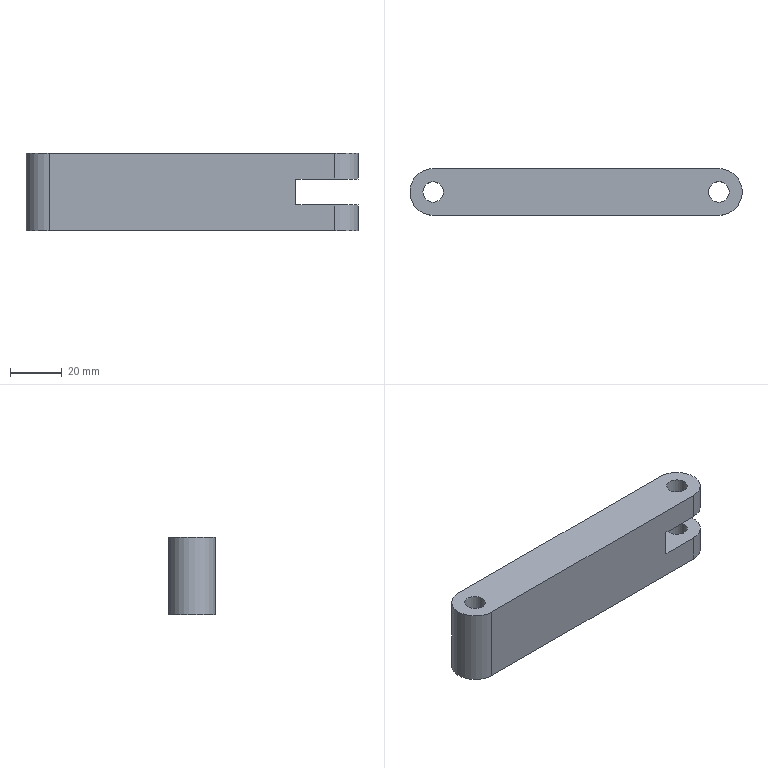Part | STEP file | 1 solid | 13 faces | box 128 x 18 x 30 mm | volume 60581 mm3 | plane 7 | cylinder 6 | commonest cylinder face diameters 18 x3 8 x2 7.914 x1
STEP:
#1=CARTESIAN_POINT('',(0.,0.,0.));
#2=DIRECTION('',(0.,0.,1.));
#3=DIRECTION('',(1.,0.,0.));
#4=AXIS2_PLACEMENT_3D('',#1,#2,#3);
#5=CARTESIAN_POINT('',(40.,-9.,-5.));
#6=VERTEX_POINT('',#5);
#7=CARTESIAN_POINT('',(55.,-9.,-5.));
#8=VERTEX_POINT('',#7);
#9=CARTESIAN_POINT('',(-55.,-9.,-5.));
#10=DIRECTION('',(1.,0.,0.));
#11=VECTOR('',#10,1.);
#12=LINE('',#9,#11);
#13=CARTESIAN_POINT('',(-55.,-9.,15.));
#14=DIRECTION('',(0.,1.,0.));
#15=DIRECTION('',(0.,0.,1.));
#16=AXIS2_PLACEMENT_3D('',#13,#14,#15);
#17=PLANE('',#16);
#18=CARTESIAN_POINT('',(-20.,0.));
#19=DIRECTION('',(0.,1.));
#20=VECTOR('',#19,1.);
#21=LINE('',#18,#20);
#22=(GEOMETRIC_REPRESENTATION_CONTEXT(2)PARAMETRIC_REPRESENTATION_CONTEXT()REPRESENTATION_CONTEXT('',''));
#23=DEFINITIONAL_REPRESENTATION('',(#21),#22);
#24=PCURVE('',#17,#23);
#25=CARTESIAN_POINT('',(0.,0.,-5.));
#26=DIRECTION('',(0.,0.,-1.));
#27=DIRECTION('',(-1.,0.,0.));
#28=AXIS2_PLACEMENT_3D('',#25,#26,#27);
#29=PLANE('',#28);
#30=CARTESIAN_POINT('',(55.,-9.));
#31=DIRECTION('',(-1.,0.));
#32=VECTOR('',#31,1.);
#33=LINE('',#30,#32);
#34=(GEOMETRIC_REPRESENTATION_CONTEXT(2)PARAMETRIC_REPRESENTATION_CONTEXT()REPRESENTATION_CONTEXT('',''));
#35=DEFINITIONAL_REPRESENTATION('',(#33),#34);
#36=PCURVE('',#29,#35);
#37=SURFACE_CURVE('',#12,(#24,#36),.PCURVE_S1.);
#38=EDGE_CURVE('',#6,#8,#37,.T.);
#39=ORIENTED_EDGE('',*,*,#38,.F.);
#40=CARTESIAN_POINT('',(40.,-9.,5.));
#41=VERTEX_POINT('',#40);
#42=CARTESIAN_POINT('',(40.,-9.,15.));
#43=DIRECTION('',(0.,0.,-1.));
#44=VECTOR('',#43,1.);
#45=LINE('',#42,#44);
#46=CARTESIAN_POINT('',(0.,95.));
#47=DIRECTION('',(-1.,0.));
#48=VECTOR('',#47,1.);
#49=LINE('',#46,#48);
#50=(GEOMETRIC_REPRESENTATION_CONTEXT(2)PARAMETRIC_REPRESENTATION_CONTEXT()REPRESENTATION_CONTEXT('',''));
#51=DEFINITIONAL_REPRESENTATION('',(#49),#50);
#52=PCURVE('',#17,#51);
#53=CARTESIAN_POINT('',(40.,-9.,-5.));
#54=DIRECTION('',(-1.,0.,0.));
#55=DIRECTION('',(0.,0.,1.));
#56=AXIS2_PLACEMENT_3D('',#53,#54,#55);
#57=PLANE('',#56);
#58=CARTESIAN_POINT('',(20.,0.));
#59=DIRECTION('',(-1.,0.));
#60=VECTOR('',#59,1.);
#61=LINE('',#58,#60);
#62=(GEOMETRIC_REPRESENTATION_CONTEXT(2)PARAMETRIC_REPRESENTATION_CONTEXT()REPRESENTATION_CONTEXT('',''));
#63=DEFINITIONAL_REPRESENTATION('',(#61),#62);
#64=PCURVE('',#57,#63);
#65=SURFACE_CURVE('',#45,(#52,#64),.PCURVE_S1.);
#66=EDGE_CURVE('',#41,#6,#65,.T.);
#67=ORIENTED_EDGE('',*,*,#66,.F.);
#68=CARTESIAN_POINT('',(55.,-9.,5.));
#69=VERTEX_POINT('',#68);
#70=CARTESIAN_POINT('',(-55.,-9.,5.));
#71=DIRECTION('',(-1.,0.,0.));
#72=VECTOR('',#71,1.);
#73=LINE('',#70,#72);
#74=CARTESIAN_POINT('',(-10.,0.));
#75=DIRECTION('',(0.,-1.));
#76=VECTOR('',#75,1.);
#77=LINE('',#74,#76);
#78=(GEOMETRIC_REPRESENTATION_CONTEXT(2)PARAMETRIC_REPRESENTATION_CONTEXT()REPRESENTATION_CONTEXT('',''));
#79=DEFINITIONAL_REPRESENTATION('',(#77),#78);
#80=PCURVE('',#17,#79);
#81=CARTESIAN_POINT('',(0.,0.,5.));
#82=DIRECTION('',(0.,0.,-1.));
#83=DIRECTION('',(-1.,0.,0.));
#84=AXIS2_PLACEMENT_3D('',#81,#82,#83);
#85=PLANE('',#84);
#86=CARTESIAN_POINT('',(55.,-9.));
#87=DIRECTION('',(1.,0.));
#88=VECTOR('',#87,1.);
#89=LINE('',#86,#88);
#90=(GEOMETRIC_REPRESENTATION_CONTEXT(2)PARAMETRIC_REPRESENTATION_CONTEXT()REPRESENTATION_CONTEXT('',''));
#91=DEFINITIONAL_REPRESENTATION('',(#89),#90);
#92=PCURVE('',#85,#91);
#93=SURFACE_CURVE('',#73,(#80,#92),.PCURVE_S1.);
#94=EDGE_CURVE('',#69,#41,#93,.T.);
#95=ORIENTED_EDGE('',*,*,#94,.F.);
#96=CARTESIAN_POINT('',(55.,-9.,15.));
#97=VERTEX_POINT('',#96);
#98=CARTESIAN_POINT('',(55.,-9.,15.));
#99=DIRECTION('',(0.,0.,-1.));
#100=VECTOR('',#99,1.);
#101=LINE('',#98,#100);
#102=CARTESIAN_POINT('',(0.,110.));
#103=DIRECTION('',(-1.,0.));
#104=VECTOR('',#103,1.);
#105=LINE('',#102,#104);
#106=(GEOMETRIC_REPRESENTATION_CONTEXT(2)PARAMETRIC_REPRESENTATION_CONTEXT()REPRESENTATION_CONTEXT('',''));
#107=DEFINITIONAL_REPRESENTATION('',(#105),#106);
#108=PCURVE('',#17,#107);
#109=CARTESIAN_POINT('',(55.,0.,15.));
#110=DIRECTION('',(0.,0.,-1.));
#111=DIRECTION('',(-1.,0.,0.));
#112=AXIS2_PLACEMENT_3D('',#109,#110,#111);
#113=CYLINDRICAL_SURFACE('',#112,9.);
#114=CARTESIAN_POINT('',(4.712,0.));
#115=DIRECTION('',(0.,1.));
#116=VECTOR('',#115,1.);
#117=LINE('',#114,#116);
#118=(GEOMETRIC_REPRESENTATION_CONTEXT(2)PARAMETRIC_REPRESENTATION_CONTEXT()REPRESENTATION_CONTEXT('',''));
#119=DEFINITIONAL_REPRESENTATION('',(#117),#118);
#120=PCURVE('',#113,#119);
#121=SURFACE_CURVE('',#101,(#108,#120),.PCURVE_S1.);
#122=EDGE_CURVE('',#97,#69,#121,.T.);
#123=ORIENTED_EDGE('',*,*,#122,.F.);
#124=CARTESIAN_POINT('',(-55.,-9.,15.));
#125=VERTEX_POINT('',#124);
#126=CARTESIAN_POINT('',(-55.,-9.,15.));
#127=DIRECTION('',(1.,0.,0.));
#128=VECTOR('',#127,1.);
#129=LINE('',#126,#128);
#130=CARTESIAN_POINT('',(0.,0.));
#131=DIRECTION('',(0.,1.));
#132=VECTOR('',#131,1.);
#133=LINE('',#130,#132);
#134=(GEOMETRIC_REPRESENTATION_CONTEXT(2)PARAMETRIC_REPRESENTATION_CONTEXT()REPRESENTATION_CONTEXT('',''));
#135=DEFINITIONAL_REPRESENTATION('',(#133),#134);
#136=PCURVE('',#17,#135);
#137=CARTESIAN_POINT('',(-55.,0.,15.));
#138=DIRECTION('',(0.,0.,1.));
#139=DIRECTION('',(1.,0.,0.));
#140=AXIS2_PLACEMENT_3D('',#137,#138,#139);
#141=PLANE('',#140);
#142=CARTESIAN_POINT('',(0.,-9.));
#143=DIRECTION('',(1.,0.));
#144=VECTOR('',#143,1.);
#145=LINE('',#142,#144);
#146=(GEOMETRIC_REPRESENTATION_CONTEXT(2)PARAMETRIC_REPRESENTATION_CONTEXT()REPRESENTATION_CONTEXT('',''));
#147=DEFINITIONAL_REPRESENTATION('',(#145),#146);
#148=PCURVE('',#141,#147);
#149=SURFACE_CURVE('',#129,(#136,#148),.PCURVE_S1.);
#150=EDGE_CURVE('',#125,#97,#149,.T.);
#151=ORIENTED_EDGE('',*,*,#150,.F.);
#152=CARTESIAN_POINT('',(-55.,-9.,-15.));
#153=VERTEX_POINT('',#152);
#154=CARTESIAN_POINT('',(-55.,-9.,15.));
#155=DIRECTION('',(0.,0.,1.));
#156=VECTOR('',#155,1.);
#157=LINE('',#154,#156);
#158=CARTESIAN_POINT('',(0.,0.));
#159=DIRECTION('',(1.,0.));
#160=VECTOR('',#159,1.);
#161=LINE('',#158,#160);
#162=(GEOMETRIC_REPRESENTATION_CONTEXT(2)PARAMETRIC_REPRESENTATION_CONTEXT()REPRESENTATION_CONTEXT('',''));
#163=DEFINITIONAL_REPRESENTATION('',(#161),#162);
#164=PCURVE('',#17,#163);
#165=CARTESIAN_POINT('',(-55.,0.,15.));
#166=DIRECTION('',(0.,0.,-1.));
#167=DIRECTION('',(-1.,0.,0.));
#168=AXIS2_PLACEMENT_3D('',#165,#166,#167);
#169=CYLINDRICAL_SURFACE('',#168,9.);
#170=CARTESIAN_POINT('',(-1.571,0.));
#171=DIRECTION('',(0.,-1.));
#172=VECTOR('',#171,1.);
#173=LINE('',#170,#172);
#174=(GEOMETRIC_REPRESENTATION_CONTEXT(2)PARAMETRIC_REPRESENTATION_CONTEXT()REPRESENTATION_CONTEXT('',''));
#175=DEFINITIONAL_REPRESENTATION('',(#173),#174);
#176=PCURVE('',#169,#175);
#177=SURFACE_CURVE('',#157,(#164,#176),.PCURVE_S1.);
#178=EDGE_CURVE('',#153,#125,#177,.T.);
#179=ORIENTED_EDGE('',*,*,#178,.F.);
#180=CARTESIAN_POINT('',(55.,-9.,-15.));
#181=VERTEX_POINT('',#180);
#182=CARTESIAN_POINT('',(-55.,-9.,-15.));
#183=DIRECTION('',(-1.,0.,0.));
#184=VECTOR('',#183,1.);
#185=LINE('',#182,#184);
#186=CARTESIAN_POINT('',(-30.,0.));
#187=DIRECTION('',(0.,-1.));
#188=VECTOR('',#187,1.);
#189=LINE('',#186,#188);
#190=(GEOMETRIC_REPRESENTATION_CONTEXT(2)PARAMETRIC_REPRESENTATION_CONTEXT()REPRESENTATION_CONTEXT('',''));
#191=DEFINITIONAL_REPRESENTATION('',(#189),#190);
#192=PCURVE('',#17,#191);
#193=CARTESIAN_POINT('',(-55.,0.,-15.));
#194=DIRECTION('',(0.,0.,1.));
#195=DIRECTION('',(1.,0.,0.));
#196=AXIS2_PLACEMENT_3D('',#193,#194,#195);
#197=PLANE('',#196);
#198=CARTESIAN_POINT('',(0.,-9.));
#199=DIRECTION('',(-1.,0.));
#200=VECTOR('',#199,1.);
#201=LINE('',#198,#200);
#202=(GEOMETRIC_REPRESENTATION_CONTEXT(2)PARAMETRIC_REPRESENTATION_CONTEXT()REPRESENTATION_CONTEXT('',''));
#203=DEFINITIONAL_REPRESENTATION('',(#201),#202);
#204=PCURVE('',#197,#203);
#205=SURFACE_CURVE('',#185,(#192,#204),.PCURVE_S1.);
#206=EDGE_CURVE('',#181,#153,#205,.T.);
#207=ORIENTED_EDGE('',*,*,#206,.F.);
#208=CARTESIAN_POINT('',(55.,-9.,15.));
#209=DIRECTION('',(0.,0.,-1.));
#210=VECTOR('',#209,1.);
#211=LINE('',#208,#210);
#212=CARTESIAN_POINT('',(0.,110.));
#213=DIRECTION('',(-1.,0.));
#214=VECTOR('',#213,1.);
#215=LINE('',#212,#214);
#216=(GEOMETRIC_REPRESENTATION_CONTEXT(2)PARAMETRIC_REPRESENTATION_CONTEXT()REPRESENTATION_CONTEXT('',''));
#217=DEFINITIONAL_REPRESENTATION('',(#215),#216);
#218=PCURVE('',#17,#217);
#219=CARTESIAN_POINT('',(55.,0.,15.));
#220=DIRECTION('',(0.,0.,-1.));
#221=DIRECTION('',(-1.,0.,0.));
#222=AXIS2_PLACEMENT_3D('',#219,#220,#221);
#223=CYLINDRICAL_SURFACE('',#222,9.);
#224=CARTESIAN_POINT('',(4.712,0.));
#225=DIRECTION('',(0.,1.));
#226=VECTOR('',#225,1.);
#227=LINE('',#224,#226);
#228=(GEOMETRIC_REPRESENTATION_CONTEXT(2)PARAMETRIC_REPRESENTATION_CONTEXT()REPRESENTATION_CONTEXT('',''));
#229=DEFINITIONAL_REPRESENTATION('',(#227),#228);
#230=PCURVE('',#223,#229);
#231=SURFACE_CURVE('',#211,(#218,#230),.PCURVE_S1.);
#232=EDGE_CURVE('',#8,#181,#231,.T.);
#233=ORIENTED_EDGE('',*,*,#232,.F.);
#234=EDGE_LOOP('',(#39,#67,#95,#123,#151,#179,#207,#233));
#235=FACE_BOUND('',#234,.T.);
#236=ADVANCED_FACE('',(#235),#17,.F.);
#237=ORIENTED_EDGE('',*,*,#232,.T.);
#238=CARTESIAN_POINT('',(55.,9.,-15.));
#239=VERTEX_POINT('',#238);
#240=CARTESIAN_POINT('',(55.,0.,-15.));
#241=DIRECTION('',(0.,0.,1.));
#242=DIRECTION('',(-1.,0.,0.));
#243=AXIS2_PLACEMENT_3D('',#240,#241,#242);
#244=CIRCLE('',#243,9.);
#245=CARTESIAN_POINT('',(6.283,30.));
#246=DIRECTION('',(-1.,0.));
#247=VECTOR('',#246,1.);
#248=LINE('',#245,#247);
#249=(GEOMETRIC_REPRESENTATION_CONTEXT(2)PARAMETRIC_REPRESENTATION_CONTEXT()REPRESENTATION_CONTEXT('',''));
#250=DEFINITIONAL_REPRESENTATION('',(#248),#249);
#251=PCURVE('',#223,#250);
#252=CARTESIAN_POINT('',(110.,0.));
#253=DIRECTION('',(-1.,0.));
#254=AXIS2_PLACEMENT_2D('',#252,#253);
#255=CIRCLE('',#254,9.);
#256=(GEOMETRIC_REPRESENTATION_CONTEXT(2)PARAMETRIC_REPRESENTATION_CONTEXT()REPRESENTATION_CONTEXT('',''));
#257=DEFINITIONAL_REPRESENTATION('',(#255),#256);
#258=PCURVE('',#197,#257);
#259=SURFACE_CURVE('',#244,(#251,#258),.PCURVE_S1.);
#260=EDGE_CURVE('',#181,#239,#259,.T.);
#261=ORIENTED_EDGE('',*,*,#260,.T.);
#262=CARTESIAN_POINT('',(55.,9.,-5.));
#263=VERTEX_POINT('',#262);
#264=CARTESIAN_POINT('',(55.,9.,15.));
#265=DIRECTION('',(0.,0.,1.));
#266=VECTOR('',#265,1.);
#267=LINE('',#264,#266);
#268=CARTESIAN_POINT('',(1.571,0.));
#269=DIRECTION('',(0.,-1.));
#270=VECTOR('',#269,1.);
#271=LINE('',#268,#270);
#272=(GEOMETRIC_REPRESENTATION_CONTEXT(2)PARAMETRIC_REPRESENTATION_CONTEXT()REPRESENTATION_CONTEXT('',''));
#273=DEFINITIONAL_REPRESENTATION('',(#271),#272);
#274=PCURVE('',#223,#273);
#275=CARTESIAN_POINT('',(-55.,9.,15.));
#276=DIRECTION('',(0.,-1.,0.));
#277=DIRECTION('',(0.,0.,-1.));
#278=AXIS2_PLACEMENT_3D('',#275,#276,#277);
#279=PLANE('',#278);
#280=CARTESIAN_POINT('',(0.,110.));
#281=DIRECTION('',(-1.,0.));
#282=VECTOR('',#281,1.);
#283=LINE('',#280,#282);
#284=(GEOMETRIC_REPRESENTATION_CONTEXT(2)PARAMETRIC_REPRESENTATION_CONTEXT()REPRESENTATION_CONTEXT('',''));
#285=DEFINITIONAL_REPRESENTATION('',(#283),#284);
#286=PCURVE('',#279,#285);
#287=SURFACE_CURVE('',#267,(#274,#286),.PCURVE_S1.);
#288=EDGE_CURVE('',#239,#263,#287,.T.);
#289=ORIENTED_EDGE('',*,*,#288,.T.);
#290=CARTESIAN_POINT('',(55.,0.,-5.));
#291=DIRECTION('',(0.,0.,-1.));
#292=DIRECTION('',(-1.,0.,0.));
#293=AXIS2_PLACEMENT_3D('',#290,#291,#292);
#294=CIRCLE('',#293,9.);
#295=CARTESIAN_POINT('',(0.,20.));
#296=DIRECTION('',(1.,0.));
#297=VECTOR('',#296,1.);
#298=LINE('',#295,#297);
#299=(GEOMETRIC_REPRESENTATION_CONTEXT(2)PARAMETRIC_REPRESENTATION_CONTEXT()REPRESENTATION_CONTEXT('',''));
#300=DEFINITIONAL_REPRESENTATION('',(#298),#299);
#301=PCURVE('',#223,#300);
#302=CARTESIAN_POINT('',(-55.,0.));
#303=DIRECTION('',(1.,0.));
#304=AXIS2_PLACEMENT_2D('',#302,#303);
#305=CIRCLE('',#304,9.);
#306=(GEOMETRIC_REPRESENTATION_CONTEXT(2)PARAMETRIC_REPRESENTATION_CONTEXT()REPRESENTATION_CONTEXT('',''));
#307=DEFINITIONAL_REPRESENTATION('',(#305),#306);
#308=PCURVE('',#29,#307);
#309=SURFACE_CURVE('',#294,(#301,#308),.PCURVE_S1.);
#310=EDGE_CURVE('',#263,#8,#309,.T.);
#311=ORIENTED_EDGE('',*,*,#310,.T.);
#312=EDGE_LOOP('',(#237,#261,#289,#311));
#313=FACE_BOUND('',#312,.T.);
#314=ADVANCED_FACE('',(#313),#223,.T.);
#315=CARTESIAN_POINT('',(51.,0.,-5.));
#316=VERTEX_POINT('',#315);
#317=CARTESIAN_POINT('',(55.,0.,-5.));
#318=DIRECTION('',(0.,0.,1.));
#319=DIRECTION('',(-1.,0.,0.));
#320=AXIS2_PLACEMENT_3D('',#317,#318,#319);
#321=CIRCLE('',#320,4.);
#322=CARTESIAN_POINT('',(-51.,0.));
#323=CARTESIAN_POINT('',(-51.,-6.928));
#324=CARTESIAN_POINT('',(-57.,-3.464));
#325=CARTESIAN_POINT('',(-63.,0.));
#326=CARTESIAN_POINT('',(-57.,3.464));
#327=CARTESIAN_POINT('',(-51.,6.928));
#328=CARTESIAN_POINT('',(-51.,0.));
#329=(BOUNDED_CURVE()B_SPLINE_CURVE(2,(#322,#323,#324,#325,#326,#327,#328),.UNSPECIFIED.,.T.,.F.)B_SPLINE_CURVE_WITH_KNOTS((1,2,2,2,2,1),(-2.094,0.,2.094,4.189,6.283,8.378),.UNSPECIFIED.)CURVE()GEOMETRIC_REPRESENTATION_ITEM()RATIONAL_B_SPLINE_CURVE((1.,0.5,1.,0.5,1.,0.5,1.))REPRESENTATION_ITEM(''));
#330=(GEOMETRIC_REPRESENTATION_CONTEXT(2)PARAMETRIC_REPRESENTATION_CONTEXT()REPRESENTATION_CONTEXT('',''));
#331=DEFINITIONAL_REPRESENTATION('',(#329),#330);
#332=PCURVE('',#29,#331);
#333=CARTESIAN_POINT('',(55.,0.,15.));
#334=DIRECTION('',(0.,0.,-1.));
#335=DIRECTION('',(-1.,0.,0.));
#336=AXIS2_PLACEMENT_3D('',#333,#334,#335);
#337=CYLINDRICAL_SURFACE('',#336,4.);
#338=CARTESIAN_POINT('',(6.283,20.));
#339=DIRECTION('',(-1.,0.));
#340=VECTOR('',#339,1.);
#341=LINE('',#338,#340);
#342=(GEOMETRIC_REPRESENTATION_CONTEXT(2)PARAMETRIC_REPRESENTATION_CONTEXT()REPRESENTATION_CONTEXT('',''));
#343=DEFINITIONAL_REPRESENTATION('',(#341),#342);
#344=PCURVE('',#337,#343);
#345=SURFACE_CURVE('',#321,(#332,#344),.PCURVE_S1.);
#346=EDGE_CURVE('',#316,#316,#345,.T.);
#347=ORIENTED_EDGE('',*,*,#346,.F.);
#348=EDGE_LOOP('',(#347));
#349=FACE_BOUND('',#348,.T.);
#350=CARTESIAN_POINT('',(40.,9.,-5.));
#351=VERTEX_POINT('',#350);
#352=CARTESIAN_POINT('',(40.,0.,-5.));
#353=DIRECTION('',(0.,1.,0.));
#354=VECTOR('',#353,1.);
#355=LINE('',#352,#354);
#356=CARTESIAN_POINT('',(-40.,0.));
#357=DIRECTION('',(0.,1.));
#358=VECTOR('',#357,1.);
#359=LINE('',#356,#358);
#360=(GEOMETRIC_REPRESENTATION_CONTEXT(2)PARAMETRIC_REPRESENTATION_CONTEXT()REPRESENTATION_CONTEXT('',''));
#361=DEFINITIONAL_REPRESENTATION('',(#359),#360);
#362=PCURVE('',#29,#361);
#363=CARTESIAN_POINT('',(0.,9.));
#364=DIRECTION('',(0.,1.));
#365=VECTOR('',#364,1.);
#366=LINE('',#363,#365);
#367=(GEOMETRIC_REPRESENTATION_CONTEXT(2)PARAMETRIC_REPRESENTATION_CONTEXT()REPRESENTATION_CONTEXT('',''));
#368=DEFINITIONAL_REPRESENTATION('',(#366),#367);
#369=PCURVE('',#57,#368);
#370=SURFACE_CURVE('',#355,(#362,#369),.PCURVE_S1.);
#371=EDGE_CURVE('',#6,#351,#370,.T.);
#372=ORIENTED_EDGE('',*,*,#371,.F.);
#373=ORIENTED_EDGE('',*,*,#38,.T.);
#374=ORIENTED_EDGE('',*,*,#310,.F.);
#375=CARTESIAN_POINT('',(0.,9.,-5.));
#376=DIRECTION('',(1.,0.,0.));
#377=VECTOR('',#376,1.);
#378=LINE('',#375,#377);
#379=CARTESIAN_POINT('',(0.,9.));
#380=DIRECTION('',(-1.,0.));
#381=VECTOR('',#380,1.);
#382=LINE('',#379,#381);
#383=(GEOMETRIC_REPRESENTATION_CONTEXT(2)PARAMETRIC_REPRESENTATION_CONTEXT()REPRESENTATION_CONTEXT('',''));
#384=DEFINITIONAL_REPRESENTATION('',(#382),#383);
#385=PCURVE('',#29,#384);
#386=CARTESIAN_POINT('',(20.,55.));
#387=DIRECTION('',(0.,1.));
#388=VECTOR('',#387,1.);
#389=LINE('',#386,#388);
#390=(GEOMETRIC_REPRESENTATION_CONTEXT(2)PARAMETRIC_REPRESENTATION_CONTEXT()REPRESENTATION_CONTEXT('',''));
#391=DEFINITIONAL_REPRESENTATION('',(#389),#390);
#392=PCURVE('',#279,#391);
#393=SURFACE_CURVE('',#378,(#385,#392),.PCURVE_S1.);
#394=EDGE_CURVE('',#351,#263,#393,.T.);
#395=ORIENTED_EDGE('',*,*,#394,.F.);
#396=EDGE_LOOP('',(#372,#373,#374,#395));
#397=FACE_BOUND('',#396,.T.);
#398=ADVANCED_FACE('',(#349,#397),#29,.F.);
#399=ORIENTED_EDGE('',*,*,#66,.T.);
#400=ORIENTED_EDGE('',*,*,#371,.T.);
#401=CARTESIAN_POINT('',(40.,9.,5.));
#402=VERTEX_POINT('',#401);
#403=CARTESIAN_POINT('',(40.,9.,-5.));
#404=DIRECTION('',(0.,0.,-1.));
#405=VECTOR('',#404,1.);
#406=LINE('',#403,#405);
#407=CARTESIAN_POINT('',(0.,18.));
#408=DIRECTION('',(-1.,0.));
#409=VECTOR('',#408,1.);
#410=LINE('',#407,#409);
#411=(GEOMETRIC_REPRESENTATION_CONTEXT(2)PARAMETRIC_REPRESENTATION_CONTEXT()REPRESENTATION_CONTEXT('',''));
#412=DEFINITIONAL_REPRESENTATION('',(#410),#411);
#413=PCURVE('',#57,#412);
#414=CARTESIAN_POINT('',(20.,95.));
#415=DIRECTION('',(1.,0.));
#416=VECTOR('',#415,1.);
#417=LINE('',#414,#416);
#418=(GEOMETRIC_REPRESENTATION_CONTEXT(2)PARAMETRIC_REPRESENTATION_CONTEXT()REPRESENTATION_CONTEXT('',''));
#419=DEFINITIONAL_REPRESENTATION('',(#417),#418);
#420=PCURVE('',#279,#419);
#421=SURFACE_CURVE('',#406,(#413,#420),.PCURVE_S1.);
#422=EDGE_CURVE('',#402,#351,#421,.T.);
#423=ORIENTED_EDGE('',*,*,#422,.F.);
#424=CARTESIAN_POINT('',(40.,-9.,5.));
#425=DIRECTION('',(0.,1.,0.));
#426=VECTOR('',#425,1.);
#427=LINE('',#424,#426);
#428=CARTESIAN_POINT('',(10.,0.));
#429=DIRECTION('',(0.,1.));
#430=VECTOR('',#429,1.);
#431=LINE('',#428,#430);
#432=(GEOMETRIC_REPRESENTATION_CONTEXT(2)PARAMETRIC_REPRESENTATION_CONTEXT()REPRESENTATION_CONTEXT('',''));
#433=DEFINITIONAL_REPRESENTATION('',(#431),#432);
#434=PCURVE('',#57,#433);
#435=CARTESIAN_POINT('',(-40.,-9.));
#436=DIRECTION('',(0.,1.));
#437=VECTOR('',#436,1.);
#438=LINE('',#435,#437);
#439=(GEOMETRIC_REPRESENTATION_CONTEXT(2)PARAMETRIC_REPRESENTATION_CONTEXT()REPRESENTATION_CONTEXT('',''));
#440=DEFINITIONAL_REPRESENTATION('',(#438),#439);
#441=PCURVE('',#85,#440);
#442=SURFACE_CURVE('',#427,(#434,#441),.PCURVE_S1.);
#443=EDGE_CURVE('',#41,#402,#442,.T.);
#444=ORIENTED_EDGE('',*,*,#443,.F.);
#445=EDGE_LOOP('',(#399,#400,#423,#444));
#446=FACE_BOUND('',#445,.T.);
#447=ADVANCED_FACE('',(#446),#57,.F.);
#448=CARTESIAN_POINT('',(51.,0.,5.));
#449=VERTEX_POINT('',#448);
#450=CARTESIAN_POINT('',(55.,0.,5.));
#451=DIRECTION('',(0.,0.,1.));
#452=DIRECTION('',(-1.,0.,0.));
#453=AXIS2_PLACEMENT_3D('',#450,#451,#452);
#454=CIRCLE('',#453,4.);
#455=CARTESIAN_POINT('',(-51.,0.));
#456=CARTESIAN_POINT('',(-51.,-6.928));
#457=CARTESIAN_POINT('',(-57.,-3.464));
#458=CARTESIAN_POINT('',(-63.,0.));
#459=CARTESIAN_POINT('',(-57.,3.464));
#460=CARTESIAN_POINT('',(-51.,6.928));
#461=CARTESIAN_POINT('',(-51.,0.));
#462=(BOUNDED_CURVE()B_SPLINE_CURVE(2,(#455,#456,#457,#458,#459,#460,#461),.UNSPECIFIED.,.T.,.F.)B_SPLINE_CURVE_WITH_KNOTS((1,2,2,2,2,1),(-2.094,0.,2.094,4.189,6.283,8.378),.UNSPECIFIED.)CURVE()GEOMETRIC_REPRESENTATION_ITEM()RATIONAL_B_SPLINE_CURVE((1.,0.5,1.,0.5,1.,0.5,1.))REPRESENTATION_ITEM(''));
#463=(GEOMETRIC_REPRESENTATION_CONTEXT(2)PARAMETRIC_REPRESENTATION_CONTEXT()REPRESENTATION_CONTEXT('',''));
#464=DEFINITIONAL_REPRESENTATION('',(#462),#463);
#465=PCURVE('',#85,#464);
#466=CARTESIAN_POINT('',(55.,0.,15.));
#467=DIRECTION('',(0.,0.,-1.));
#468=DIRECTION('',(-1.,0.,0.));
#469=AXIS2_PLACEMENT_3D('',#466,#467,#468);
#470=CYLINDRICAL_SURFACE('',#469,4.);
#471=CARTESIAN_POINT('',(6.283,10.));
#472=DIRECTION('',(-1.,0.));
#473=VECTOR('',#472,1.);
#474=LINE('',#471,#473);
#475=(GEOMETRIC_REPRESENTATION_CONTEXT(2)PARAMETRIC_REPRESENTATION_CONTEXT()REPRESENTATION_CONTEXT('',''));
#476=DEFINITIONAL_REPRESENTATION('',(#474),#475);
#477=PCURVE('',#470,#476);
#478=SURFACE_CURVE('',#454,(#465,#477),.PCURVE_S1.);
#479=EDGE_CURVE('',#449,#449,#478,.T.);
#480=ORIENTED_EDGE('',*,*,#479,.T.);
#481=EDGE_LOOP('',(#480));
#482=FACE_BOUND('',#481,.T.);
#483=ORIENTED_EDGE('',*,*,#443,.T.);
#484=CARTESIAN_POINT('',(55.,9.,5.));
#485=VERTEX_POINT('',#484);
#486=CARTESIAN_POINT('',(0.,9.,5.));
#487=DIRECTION('',(1.,0.,0.));
#488=VECTOR('',#487,1.);
#489=LINE('',#486,#488);
#490=CARTESIAN_POINT('',(0.,9.));
#491=DIRECTION('',(-1.,0.));
#492=VECTOR('',#491,1.);
#493=LINE('',#490,#492);
#494=(GEOMETRIC_REPRESENTATION_CONTEXT(2)PARAMETRIC_REPRESENTATION_CONTEXT()REPRESENTATION_CONTEXT('',''));
#495=DEFINITIONAL_REPRESENTATION('',(#493),#494);
#496=PCURVE('',#85,#495);
#497=CARTESIAN_POINT('',(10.,55.));
#498=DIRECTION('',(0.,1.));
#499=VECTOR('',#498,1.);
#500=LINE('',#497,#499);
#501=(GEOMETRIC_REPRESENTATION_CONTEXT(2)PARAMETRIC_REPRESENTATION_CONTEXT()REPRESENTATION_CONTEXT('',''));
#502=DEFINITIONAL_REPRESENTATION('',(#500),#501);
#503=PCURVE('',#279,#502);
#504=SURFACE_CURVE('',#489,(#496,#503),.PCURVE_S1.);
#505=EDGE_CURVE('',#402,#485,#504,.T.);
#506=ORIENTED_EDGE('',*,*,#505,.T.);
#507=CARTESIAN_POINT('',(55.,0.,5.));
#508=DIRECTION('',(0.,0.,-1.));
#509=DIRECTION('',(-1.,0.,0.));
#510=AXIS2_PLACEMENT_3D('',#507,#508,#509);
#511=CIRCLE('',#510,9.);
#512=CARTESIAN_POINT('',(-55.,0.));
#513=DIRECTION('',(1.,0.));
#514=AXIS2_PLACEMENT_2D('',#512,#513);
#515=CIRCLE('',#514,9.);
#516=(GEOMETRIC_REPRESENTATION_CONTEXT(2)PARAMETRIC_REPRESENTATION_CONTEXT()REPRESENTATION_CONTEXT('',''));
#517=DEFINITIONAL_REPRESENTATION('',(#515),#516);
#518=PCURVE('',#85,#517);
#519=CARTESIAN_POINT('',(0.,10.));
#520=DIRECTION('',(1.,0.));
#521=VECTOR('',#520,1.);
#522=LINE('',#519,#521);
#523=(GEOMETRIC_REPRESENTATION_CONTEXT(2)PARAMETRIC_REPRESENTATION_CONTEXT()REPRESENTATION_CONTEXT('',''));
#524=DEFINITIONAL_REPRESENTATION('',(#522),#523);
#525=PCURVE('',#113,#524);
#526=SURFACE_CURVE('',#511,(#518,#525),.PCURVE_S1.);
#527=EDGE_CURVE('',#485,#69,#526,.T.);
#528=ORIENTED_EDGE('',*,*,#527,.T.);
#529=ORIENTED_EDGE('',*,*,#94,.T.);
#530=EDGE_LOOP('',(#483,#506,#528,#529));
#531=FACE_BOUND('',#530,.T.);
#532=ADVANCED_FACE('',(#482,#531),#85,.T.);
#533=CARTESIAN_POINT('',(55.,9.,15.));
#534=VERTEX_POINT('',#533);
#535=CARTESIAN_POINT('',(55.,0.,15.));
#536=DIRECTION('',(0.,0.,-1.));
#537=DIRECTION('',(-1.,0.,0.));
#538=AXIS2_PLACEMENT_3D('',#535,#536,#537);
#539=CIRCLE('',#538,9.);
#540=CARTESIAN_POINT('',(0.,0.));
#541=DIRECTION('',(1.,0.));
#542=VECTOR('',#541,1.);
#543=LINE('',#540,#542);
#544=(GEOMETRIC_REPRESENTATION_CONTEXT(2)PARAMETRIC_REPRESENTATION_CONTEXT()REPRESENTATION_CONTEXT('',''));
#545=DEFINITIONAL_REPRESENTATION('',(#543),#544);
#546=PCURVE('',#113,#545);
#547=CARTESIAN_POINT('',(101.,0.));
#548=CARTESIAN_POINT('',(101.,15.588));
#549=CARTESIAN_POINT('',(114.5,7.794));
#550=CARTESIAN_POINT('',(128.,0.));
#551=CARTESIAN_POINT('',(114.5,-7.794));
#552=CARTESIAN_POINT('',(101.,-15.588));
#553=CARTESIAN_POINT('',(101.,0.));
#554=(BOUNDED_CURVE()B_SPLINE_CURVE(2,(#547,#548,#549,#550,#551,#552,#553),.UNSPECIFIED.,.T.,.F.)B_SPLINE_CURVE_WITH_KNOTS((1,2,2,2,2,1),(-2.094,0.,2.094,4.189,6.283,8.378),.UNSPECIFIED.)CURVE()GEOMETRIC_REPRESENTATION_ITEM()RATIONAL_B_SPLINE_CURVE((1.,0.5,1.,0.5,1.,0.5,1.))REPRESENTATION_ITEM(''));
#555=(GEOMETRIC_REPRESENTATION_CONTEXT(2)PARAMETRIC_REPRESENTATION_CONTEXT()REPRESENTATION_CONTEXT('',''));
#556=DEFINITIONAL_REPRESENTATION('',(#554),#555);
#557=PCURVE('',#141,#556);
#558=SURFACE_CURVE('',#539,(#546,#557),.PCURVE_S1.);
#559=EDGE_CURVE('',#534,#97,#558,.T.);
#560=ORIENTED_EDGE('',*,*,#559,.T.);
#561=ORIENTED_EDGE('',*,*,#122,.T.);
#562=ORIENTED_EDGE('',*,*,#527,.F.);
#563=CARTESIAN_POINT('',(55.,9.,15.));
#564=DIRECTION('',(0.,0.,1.));
#565=VECTOR('',#564,1.);
#566=LINE('',#563,#565);
#567=CARTESIAN_POINT('',(1.571,0.));
#568=DIRECTION('',(0.,-1.));
#569=VECTOR('',#568,1.);
#570=LINE('',#567,#569);
#571=(GEOMETRIC_REPRESENTATION_CONTEXT(2)PARAMETRIC_REPRESENTATION_CONTEXT()REPRESENTATION_CONTEXT('',''));
#572=DEFINITIONAL_REPRESENTATION('',(#570),#571);
#573=PCURVE('',#113,#572);
#574=CARTESIAN_POINT('',(0.,110.));
#575=DIRECTION('',(-1.,0.));
#576=VECTOR('',#575,1.);
#577=LINE('',#574,#576);
#578=(GEOMETRIC_REPRESENTATION_CONTEXT(2)PARAMETRIC_REPRESENTATION_CONTEXT()REPRESENTATION_CONTEXT('',''));
#579=DEFINITIONAL_REPRESENTATION('',(#577),#578);
#580=PCURVE('',#279,#579);
#581=SURFACE_CURVE('',#566,(#573,#580),.PCURVE_S1.);
#582=EDGE_CURVE('',#485,#534,#581,.T.);
#583=ORIENTED_EDGE('',*,*,#582,.T.);
#584=EDGE_LOOP('',(#560,#561,#562,#583));
#585=FACE_BOUND('',#584,.T.);
#586=ADVANCED_FACE('',(#585),#113,.T.);
#587=CARTESIAN_POINT('',(51.,0.,15.));
#588=VERTEX_POINT('',#587);
#589=CARTESIAN_POINT('',(55.,0.,15.));
#590=DIRECTION('',(0.,0.,-1.));
#591=DIRECTION('',(-1.,0.,0.));
#592=AXIS2_PLACEMENT_3D('',#589,#590,#591);
#593=CIRCLE('',#592,4.);
#594=CARTESIAN_POINT('',(106.,0.));
#595=CARTESIAN_POINT('',(106.,6.928));
#596=CARTESIAN_POINT('',(112.,3.464));
#597=CARTESIAN_POINT('',(118.,0.));
#598=CARTESIAN_POINT('',(112.,-3.464));
#599=CARTESIAN_POINT('',(106.,-6.928));
#600=CARTESIAN_POINT('',(106.,0.));
#601=(BOUNDED_CURVE()B_SPLINE_CURVE(2,(#594,#595,#596,#597,#598,#599,#600),.UNSPECIFIED.,.T.,.F.)B_SPLINE_CURVE_WITH_KNOTS((1,2,2,2,2,1),(-2.094,0.,2.094,4.189,6.283,8.378),.UNSPECIFIED.)CURVE()GEOMETRIC_REPRESENTATION_ITEM()RATIONAL_B_SPLINE_CURVE((1.,0.5,1.,0.5,1.,0.5,1.))REPRESENTATION_ITEM(''));
#602=(GEOMETRIC_REPRESENTATION_CONTEXT(2)PARAMETRIC_REPRESENTATION_CONTEXT()REPRESENTATION_CONTEXT('',''));
#603=DEFINITIONAL_REPRESENTATION('',(#601),#602);
#604=PCURVE('',#141,#603);
#605=CARTESIAN_POINT('',(0.,0.));
#606=DIRECTION('',(1.,0.));
#607=VECTOR('',#606,1.);
#608=LINE('',#605,#607);
#609=(GEOMETRIC_REPRESENTATION_CONTEXT(2)PARAMETRIC_REPRESENTATION_CONTEXT()REPRESENTATION_CONTEXT('',''));
#610=DEFINITIONAL_REPRESENTATION('',(#608),#609);
#611=PCURVE('',#470,#610);
#612=SURFACE_CURVE('',#593,(#604,#611),.PCURVE_S1.);
#613=EDGE_CURVE('',#588,#588,#612,.T.);
#614=ORIENTED_EDGE('',*,*,#613,.T.);
#615=EDGE_LOOP('',(#614));
#616=FACE_BOUND('',#615,.T.);
#617=CARTESIAN_POINT('',(-58.957,0.,15.));
#618=VERTEX_POINT('',#617);
#619=CARTESIAN_POINT('',(-55.,0.,15.));
#620=DIRECTION('',(0.,0.,-1.));
#621=DIRECTION('',(-1.,0.,0.));
#622=AXIS2_PLACEMENT_3D('',#619,#620,#621);
#623=CIRCLE('',#622,3.957);
#624=CARTESIAN_POINT('',(-3.957,0.));
#625=CARTESIAN_POINT('',(-3.957,6.854));
#626=CARTESIAN_POINT('',(1.978,3.427));
#627=CARTESIAN_POINT('',(7.914,0.));
#628=CARTESIAN_POINT('',(1.978,-3.427));
#629=CARTESIAN_POINT('',(-3.957,-6.854));
#630=CARTESIAN_POINT('',(-3.957,0.));
#631=(BOUNDED_CURVE()B_SPLINE_CURVE(2,(#624,#625,#626,#627,#628,#629,#630),.UNSPECIFIED.,.T.,.F.)B_SPLINE_CURVE_WITH_KNOTS((1,2,2,2,2,1),(-2.094,0.,2.094,4.189,6.283,8.378),.UNSPECIFIED.)CURVE()GEOMETRIC_REPRESENTATION_ITEM()RATIONAL_B_SPLINE_CURVE((1.,0.5,1.,0.5,1.,0.5,1.))REPRESENTATION_ITEM(''));
#632=(GEOMETRIC_REPRESENTATION_CONTEXT(2)PARAMETRIC_REPRESENTATION_CONTEXT()REPRESENTATION_CONTEXT('',''));
#633=DEFINITIONAL_REPRESENTATION('',(#631),#632);
#634=PCURVE('',#141,#633);
#635=CARTESIAN_POINT('',(-55.,0.,15.));
#636=DIRECTION('',(0.,0.,-1.));
#637=DIRECTION('',(-1.,0.,0.));
#638=AXIS2_PLACEMENT_3D('',#635,#636,#637);
#639=CYLINDRICAL_SURFACE('',#638,3.957);
#640=CARTESIAN_POINT('',(0.,0.));
#641=DIRECTION('',(1.,0.));
#642=VECTOR('',#641,1.);
#643=LINE('',#640,#642);
#644=(GEOMETRIC_REPRESENTATION_CONTEXT(2)PARAMETRIC_REPRESENTATION_CONTEXT()REPRESENTATION_CONTEXT('',''));
#645=DEFINITIONAL_REPRESENTATION('',(#643),#644);
#646=PCURVE('',#639,#645);
#647=SURFACE_CURVE('',#623,(#634,#646),.PCURVE_S1.);
#648=EDGE_CURVE('',#618,#618,#647,.T.);
#649=ORIENTED_EDGE('',*,*,#648,.T.);
#650=EDGE_LOOP('',(#649));
#651=FACE_BOUND('',#650,.T.);
#652=ORIENTED_EDGE('',*,*,#559,.F.);
#653=CARTESIAN_POINT('',(-55.,9.,15.));
#654=VERTEX_POINT('',#653);
#655=CARTESIAN_POINT('',(-55.,9.,15.));
#656=DIRECTION('',(-1.,0.,0.));
#657=VECTOR('',#656,1.);
#658=LINE('',#655,#657);
#659=CARTESIAN_POINT('',(0.,9.));
#660=DIRECTION('',(-1.,0.));
#661=VECTOR('',#660,1.);
#662=LINE('',#659,#661);
#663=(GEOMETRIC_REPRESENTATION_CONTEXT(2)PARAMETRIC_REPRESENTATION_CONTEXT()REPRESENTATION_CONTEXT('',''));
#664=DEFINITIONAL_REPRESENTATION('',(#662),#663);
#665=PCURVE('',#141,#664);
#666=CARTESIAN_POINT('',(0.,0.));
#667=DIRECTION('',(0.,-1.));
#668=VECTOR('',#667,1.);
#669=LINE('',#666,#668);
#670=(GEOMETRIC_REPRESENTATION_CONTEXT(2)PARAMETRIC_REPRESENTATION_CONTEXT()REPRESENTATION_CONTEXT('',''));
#671=DEFINITIONAL_REPRESENTATION('',(#669),#670);
#672=PCURVE('',#279,#671);
#673=SURFACE_CURVE('',#658,(#665,#672),.PCURVE_S1.);
#674=EDGE_CURVE('',#534,#654,#673,.T.);
#675=ORIENTED_EDGE('',*,*,#674,.T.);
#676=CARTESIAN_POINT('',(-55.,0.,15.));
#677=DIRECTION('',(0.,0.,1.));
#678=DIRECTION('',(-1.,0.,0.));
#679=AXIS2_PLACEMENT_3D('',#676,#677,#678);
#680=CIRCLE('',#679,9.);
#681=CARTESIAN_POINT('',(0.,0.));
#682=DIRECTION('',(-1.,0.));
#683=AXIS2_PLACEMENT_2D('',#681,#682);
#684=CIRCLE('',#683,9.);
#685=(GEOMETRIC_REPRESENTATION_CONTEXT(2)PARAMETRIC_REPRESENTATION_CONTEXT()REPRESENTATION_CONTEXT('',''));
#686=DEFINITIONAL_REPRESENTATION('',(#684),#685);
#687=PCURVE('',#141,#686);
#688=CARTESIAN_POINT('',(6.283,0.));
#689=DIRECTION('',(-1.,0.));
#690=VECTOR('',#689,1.);
#691=LINE('',#688,#690);
#692=(GEOMETRIC_REPRESENTATION_CONTEXT(2)PARAMETRIC_REPRESENTATION_CONTEXT()REPRESENTATION_CONTEXT('',''));
#693=DEFINITIONAL_REPRESENTATION('',(#691),#692);
#694=PCURVE('',#169,#693);
#695=SURFACE_CURVE('',#680,(#687,#694),.PCURVE_S1.);
#696=EDGE_CURVE('',#654,#125,#695,.T.);
#697=ORIENTED_EDGE('',*,*,#696,.T.);
#698=ORIENTED_EDGE('',*,*,#150,.T.);
#699=EDGE_LOOP('',(#652,#675,#697,#698));
#700=FACE_BOUND('',#699,.T.);
#701=ADVANCED_FACE('',(#616,#651,#700),#141,.T.);
#702=CARTESIAN_POINT('',(-55.,9.,-15.));
#703=VERTEX_POINT('',#702);
#704=CARTESIAN_POINT('',(-55.,0.,-15.));
#705=DIRECTION('',(0.,0.,1.));
#706=DIRECTION('',(-1.,0.,0.));
#707=AXIS2_PLACEMENT_3D('',#704,#705,#706);
#708=CIRCLE('',#707,9.);
#709=CARTESIAN_POINT('',(6.283,30.));
#710=DIRECTION('',(-1.,0.));
#711=VECTOR('',#710,1.);
#712=LINE('',#709,#711);
#713=(GEOMETRIC_REPRESENTATION_CONTEXT(2)PARAMETRIC_REPRESENTATION_CONTEXT()REPRESENTATION_CONTEXT('',''));
#714=DEFINITIONAL_REPRESENTATION('',(#712),#713);
#715=PCURVE('',#169,#714);
#716=CARTESIAN_POINT('',(0.,0.));
#717=DIRECTION('',(-1.,0.));
#718=AXIS2_PLACEMENT_2D('',#716,#717);
#719=CIRCLE('',#718,9.);
#720=(GEOMETRIC_REPRESENTATION_CONTEXT(2)PARAMETRIC_REPRESENTATION_CONTEXT()REPRESENTATION_CONTEXT('',''));
#721=DEFINITIONAL_REPRESENTATION('',(#719),#720);
#722=PCURVE('',#197,#721);
#723=SURFACE_CURVE('',#708,(#715,#722),.PCURVE_S1.);
#724=EDGE_CURVE('',#703,#153,#723,.T.);
#725=ORIENTED_EDGE('',*,*,#724,.T.);
#726=ORIENTED_EDGE('',*,*,#178,.T.);
#727=ORIENTED_EDGE('',*,*,#696,.F.);
#728=CARTESIAN_POINT('',(-55.,9.,15.));
#729=DIRECTION('',(0.,0.,-1.));
#730=VECTOR('',#729,1.);
#731=LINE('',#728,#730);
#732=CARTESIAN_POINT('',(1.571,0.));
#733=DIRECTION('',(0.,1.));
#734=VECTOR('',#733,1.);
#735=LINE('',#732,#734);
#736=(GEOMETRIC_REPRESENTATION_CONTEXT(2)PARAMETRIC_REPRESENTATION_CONTEXT()REPRESENTATION_CONTEXT('',''));
#737=DEFINITIONAL_REPRESENTATION('',(#735),#736);
#738=PCURVE('',#169,#737);
#739=CARTESIAN_POINT('',(0.,0.));
#740=DIRECTION('',(1.,0.));
#741=VECTOR('',#740,1.);
#742=LINE('',#739,#741);
#743=(GEOMETRIC_REPRESENTATION_CONTEXT(2)PARAMETRIC_REPRESENTATION_CONTEXT()REPRESENTATION_CONTEXT('',''));
#744=DEFINITIONAL_REPRESENTATION('',(#742),#743);
#745=PCURVE('',#279,#744);
#746=SURFACE_CURVE('',#731,(#738,#745),.PCURVE_S1.);
#747=EDGE_CURVE('',#654,#703,#746,.T.);
#748=ORIENTED_EDGE('',*,*,#747,.T.);
#749=EDGE_LOOP('',(#725,#726,#727,#748));
#750=FACE_BOUND('',#749,.T.);
#751=ADVANCED_FACE('',(#750),#169,.T.);
#752=CARTESIAN_POINT('',(51.,0.,-15.));
#753=VERTEX_POINT('',#752);
#754=CARTESIAN_POINT('',(55.,0.,-15.));
#755=DIRECTION('',(0.,0.,-1.));
#756=DIRECTION('',(-1.,0.,0.));
#757=AXIS2_PLACEMENT_3D('',#754,#755,#756);
#758=CIRCLE('',#757,4.);
#759=CARTESIAN_POINT('',(106.,0.));
#760=CARTESIAN_POINT('',(106.,6.928));
#761=CARTESIAN_POINT('',(112.,3.464));
#762=CARTESIAN_POINT('',(118.,0.));
#763=CARTESIAN_POINT('',(112.,-3.464));
#764=CARTESIAN_POINT('',(106.,-6.928));
#765=CARTESIAN_POINT('',(106.,0.));
#766=(BOUNDED_CURVE()B_SPLINE_CURVE(2,(#759,#760,#761,#762,#763,#764,#765),.UNSPECIFIED.,.T.,.F.)B_SPLINE_CURVE_WITH_KNOTS((1,2,2,2,2,1),(-2.094,0.,2.094,4.189,6.283,8.378),.UNSPECIFIED.)CURVE()GEOMETRIC_REPRESENTATION_ITEM()RATIONAL_B_SPLINE_CURVE((1.,0.5,1.,0.5,1.,0.5,1.))REPRESENTATION_ITEM(''));
#767=(GEOMETRIC_REPRESENTATION_CONTEXT(2)PARAMETRIC_REPRESENTATION_CONTEXT()REPRESENTATION_CONTEXT('',''));
#768=DEFINITIONAL_REPRESENTATION('',(#766),#767);
#769=PCURVE('',#197,#768);
#770=CARTESIAN_POINT('',(0.,30.));
#771=DIRECTION('',(1.,0.));
#772=VECTOR('',#771,1.);
#773=LINE('',#770,#772);
#774=(GEOMETRIC_REPRESENTATION_CONTEXT(2)PARAMETRIC_REPRESENTATION_CONTEXT()REPRESENTATION_CONTEXT('',''));
#775=DEFINITIONAL_REPRESENTATION('',(#773),#774);
#776=PCURVE('',#337,#775);
#777=SURFACE_CURVE('',#758,(#769,#776),.PCURVE_S1.);
#778=EDGE_CURVE('',#753,#753,#777,.T.);
#779=ORIENTED_EDGE('',*,*,#778,.F.);
#780=EDGE_LOOP('',(#779));
#781=FACE_BOUND('',#780,.T.);
#782=CARTESIAN_POINT('',(-58.957,0.,-15.));
#783=VERTEX_POINT('',#782);
#784=CARTESIAN_POINT('',(-55.,0.,-15.));
#785=DIRECTION('',(0.,0.,-1.));
#786=DIRECTION('',(-1.,0.,0.));
#787=AXIS2_PLACEMENT_3D('',#784,#785,#786);
#788=CIRCLE('',#787,3.957);
#789=CARTESIAN_POINT('',(-3.957,0.));
#790=CARTESIAN_POINT('',(-3.957,6.854));
#791=CARTESIAN_POINT('',(1.978,3.427));
#792=CARTESIAN_POINT('',(7.914,0.));
#793=CARTESIAN_POINT('',(1.978,-3.427));
#794=CARTESIAN_POINT('',(-3.957,-6.854));
#795=CARTESIAN_POINT('',(-3.957,0.));
#796=(BOUNDED_CURVE()B_SPLINE_CURVE(2,(#789,#790,#791,#792,#793,#794,#795),.UNSPECIFIED.,.T.,.F.)B_SPLINE_CURVE_WITH_KNOTS((1,2,2,2,2,1),(-2.094,0.,2.094,4.189,6.283,8.378),.UNSPECIFIED.)CURVE()GEOMETRIC_REPRESENTATION_ITEM()RATIONAL_B_SPLINE_CURVE((1.,0.5,1.,0.5,1.,0.5,1.))REPRESENTATION_ITEM(''));
#797=(GEOMETRIC_REPRESENTATION_CONTEXT(2)PARAMETRIC_REPRESENTATION_CONTEXT()REPRESENTATION_CONTEXT('',''));
#798=DEFINITIONAL_REPRESENTATION('',(#796),#797);
#799=PCURVE('',#197,#798);
#800=CARTESIAN_POINT('',(0.,30.));
#801=DIRECTION('',(1.,0.));
#802=VECTOR('',#801,1.);
#803=LINE('',#800,#802);
#804=(GEOMETRIC_REPRESENTATION_CONTEXT(2)PARAMETRIC_REPRESENTATION_CONTEXT()REPRESENTATION_CONTEXT('',''));
#805=DEFINITIONAL_REPRESENTATION('',(#803),#804);
#806=PCURVE('',#639,#805);
#807=SURFACE_CURVE('',#788,(#799,#806),.PCURVE_S1.);
#808=EDGE_CURVE('',#783,#783,#807,.T.);
#809=ORIENTED_EDGE('',*,*,#808,.F.);
#810=EDGE_LOOP('',(#809));
#811=FACE_BOUND('',#810,.T.);
#812=CARTESIAN_POINT('',(-55.,9.,-15.));
#813=DIRECTION('',(-1.,0.,0.));
#814=VECTOR('',#813,1.);
#815=LINE('',#812,#814);
#816=CARTESIAN_POINT('',(0.,9.));
#817=DIRECTION('',(-1.,0.));
#818=VECTOR('',#817,1.);
#819=LINE('',#816,#818);
#820=(GEOMETRIC_REPRESENTATION_CONTEXT(2)PARAMETRIC_REPRESENTATION_CONTEXT()REPRESENTATION_CONTEXT('',''));
#821=DEFINITIONAL_REPRESENTATION('',(#819),#820);
#822=PCURVE('',#197,#821);
#823=CARTESIAN_POINT('',(30.,0.));
#824=DIRECTION('',(0.,-1.));
#825=VECTOR('',#824,1.);
#826=LINE('',#823,#825);
#827=(GEOMETRIC_REPRESENTATION_CONTEXT(2)PARAMETRIC_REPRESENTATION_CONTEXT()REPRESENTATION_CONTEXT('',''));
#828=DEFINITIONAL_REPRESENTATION('',(#826),#827);
#829=PCURVE('',#279,#828);
#830=SURFACE_CURVE('',#815,(#822,#829),.PCURVE_S1.);
#831=EDGE_CURVE('',#239,#703,#830,.T.);
#832=ORIENTED_EDGE('',*,*,#831,.F.);
#833=ORIENTED_EDGE('',*,*,#260,.F.);
#834=ORIENTED_EDGE('',*,*,#206,.T.);
#835=ORIENTED_EDGE('',*,*,#724,.F.);
#836=EDGE_LOOP('',(#832,#833,#834,#835));
#837=FACE_BOUND('',#836,.T.);
#838=ADVANCED_FACE('',(#781,#811,#837),#197,.F.);
#839=ORIENTED_EDGE('',*,*,#394,.T.);
#840=ORIENTED_EDGE('',*,*,#288,.F.);
#841=ORIENTED_EDGE('',*,*,#831,.T.);
#842=ORIENTED_EDGE('',*,*,#747,.F.);
#843=ORIENTED_EDGE('',*,*,#674,.F.);
#844=ORIENTED_EDGE('',*,*,#582,.F.);
#845=ORIENTED_EDGE('',*,*,#505,.F.);
#846=ORIENTED_EDGE('',*,*,#422,.T.);
#847=EDGE_LOOP('',(#839,#840,#841,#842,#843,#844,#845,#846));
#848=FACE_BOUND('',#847,.T.);
#849=ADVANCED_FACE('',(#848),#279,.F.);
#850=ORIENTED_EDGE('',*,*,#346,.F.);
#851=CARTESIAN_POINT('',(51.,0.,-5.));
#852=CARTESIAN_POINT('',(51.,0.,-15.));
#853=B_SPLINE_CURVE_WITH_KNOTS('',1,(#851,#852),.UNSPECIFIED.,.F.,.F.,(2,2),(20.,30.),.PIECEWISE_BEZIER_KNOTS.);
#854=CARTESIAN_POINT('',(6.283,0.));
#855=DIRECTION('',(0.,1.));
#856=VECTOR('',#855,1.);
#857=LINE('',#854,#856);
#858=(GEOMETRIC_REPRESENTATION_CONTEXT(2)PARAMETRIC_REPRESENTATION_CONTEXT()REPRESENTATION_CONTEXT('',''));
#859=DEFINITIONAL_REPRESENTATION('',(#857),#858);
#860=PCURVE('',#337,#859);
#861=CARTESIAN_POINT('',(0.,0.));
#862=DIRECTION('',(0.,1.));
#863=VECTOR('',#862,1.);
#864=LINE('',#861,#863);
#865=(GEOMETRIC_REPRESENTATION_CONTEXT(2)PARAMETRIC_REPRESENTATION_CONTEXT()REPRESENTATION_CONTEXT('',''));
#866=DEFINITIONAL_REPRESENTATION('',(#864),#865);
#867=PCURVE('',#337,#866);
#868=SEAM_CURVE('',#853,(#860,#867),.PCURVE_S1.);
#869=EDGE_CURVE('',#316,#753,#868,.T.);
#870=ORIENTED_EDGE('',*,*,#869,.T.);
#871=ORIENTED_EDGE('',*,*,#778,.F.);
#872=ORIENTED_EDGE('',*,*,#869,.F.);
#873=EDGE_LOOP('',(#850,#870,#871,#872));
#874=FACE_BOUND('',#873,.F.);
#875=ADVANCED_FACE('',(#874),#337,.F.);
#876=ORIENTED_EDGE('',*,*,#479,.T.);
#877=CARTESIAN_POINT('',(51.,0.,15.));
#878=CARTESIAN_POINT('',(51.,0.,5.));
#879=B_SPLINE_CURVE_WITH_KNOTS('',1,(#877,#878),.UNSPECIFIED.,.F.,.F.,(2,2),(0.,10.),.PIECEWISE_BEZIER_KNOTS.);
#880=CARTESIAN_POINT('',(0.,0.));
#881=DIRECTION('',(0.,1.));
#882=VECTOR('',#881,1.);
#883=LINE('',#880,#882);
#884=(GEOMETRIC_REPRESENTATION_CONTEXT(2)PARAMETRIC_REPRESENTATION_CONTEXT()REPRESENTATION_CONTEXT('',''));
#885=DEFINITIONAL_REPRESENTATION('',(#883),#884);
#886=PCURVE('',#470,#885);
#887=CARTESIAN_POINT('',(6.283,0.));
#888=DIRECTION('',(0.,1.));
#889=VECTOR('',#888,1.);
#890=LINE('',#887,#889);
#891=(GEOMETRIC_REPRESENTATION_CONTEXT(2)PARAMETRIC_REPRESENTATION_CONTEXT()REPRESENTATION_CONTEXT('',''));
#892=DEFINITIONAL_REPRESENTATION('',(#890),#891);
#893=PCURVE('',#470,#892);
#894=SEAM_CURVE('',#879,(#886,#893),.PCURVE_S1.);
#895=EDGE_CURVE('',#588,#449,#894,.T.);
#896=ORIENTED_EDGE('',*,*,#895,.F.);
#897=ORIENTED_EDGE('',*,*,#613,.T.);
#898=ORIENTED_EDGE('',*,*,#895,.T.);
#899=EDGE_LOOP('',(#876,#896,#897,#898));
#900=FACE_BOUND('',#899,.F.);
#901=ADVANCED_FACE('',(#900),#470,.F.);
#902=ORIENTED_EDGE('',*,*,#648,.T.);
#903=CARTESIAN_POINT('',(-58.957,0.,15.));
#904=CARTESIAN_POINT('',(-58.957,0.,-15.));
#905=B_SPLINE_CURVE_WITH_KNOTS('',1,(#903,#904),.UNSPECIFIED.,.F.,.F.,(2,2),(0.,30.),.PIECEWISE_BEZIER_KNOTS.);
#906=CARTESIAN_POINT('',(6.283,0.));
#907=DIRECTION('',(0.,1.));
#908=VECTOR('',#907,1.);
#909=LINE('',#906,#908);
#910=(GEOMETRIC_REPRESENTATION_CONTEXT(2)PARAMETRIC_REPRESENTATION_CONTEXT()REPRESENTATION_CONTEXT('',''));
#911=DEFINITIONAL_REPRESENTATION('',(#909),#910);
#912=PCURVE('',#639,#911);
#913=CARTESIAN_POINT('',(0.,0.));
#914=DIRECTION('',(0.,1.));
#915=VECTOR('',#914,1.);
#916=LINE('',#913,#915);
#917=(GEOMETRIC_REPRESENTATION_CONTEXT(2)PARAMETRIC_REPRESENTATION_CONTEXT()REPRESENTATION_CONTEXT('',''));
#918=DEFINITIONAL_REPRESENTATION('',(#916),#917);
#919=PCURVE('',#639,#918);
#920=SEAM_CURVE('',#905,(#912,#919),.PCURVE_S1.);
#921=EDGE_CURVE('',#618,#783,#920,.T.);
#922=ORIENTED_EDGE('',*,*,#921,.T.);
#923=ORIENTED_EDGE('',*,*,#808,.F.);
#924=ORIENTED_EDGE('',*,*,#921,.F.);
#925=EDGE_LOOP('',(#902,#922,#923,#924));
#926=FACE_BOUND('',#925,.F.);
#927=ADVANCED_FACE('',(#926),#639,.F.);
#928=CLOSED_SHELL('',(#236,#314,#398,#447,#532,#586,#701,#751,#838,#849,#875,#901,#927));
#929=MANIFOLD_SOLID_BREP('',#928);
#930=(LENGTH_UNIT()NAMED_UNIT(*)SI_UNIT(.MILLI.,.METRE.));
#931=UNCERTAINTY_MEASURE_WITH_UNIT(LENGTH_MEASURE(0.000002),#930,'','');
#932=(NAMED_UNIT(*)PLANE_ANGLE_UNIT()SI_UNIT($,.RADIAN.));
#933=(NAMED_UNIT(*)SI_UNIT($,.STERADIAN.)SOLID_ANGLE_UNIT());
#934=(GEOMETRIC_REPRESENTATION_CONTEXT(3)GLOBAL_UNCERTAINTY_ASSIGNED_CONTEXT((#931))GLOBAL_UNIT_ASSIGNED_CONTEXT((#930,#932,#933))REPRESENTATION_CONTEXT('',''));
#935=ADVANCED_BREP_SHAPE_REPRESENTATION('',(#4,#929),#934);